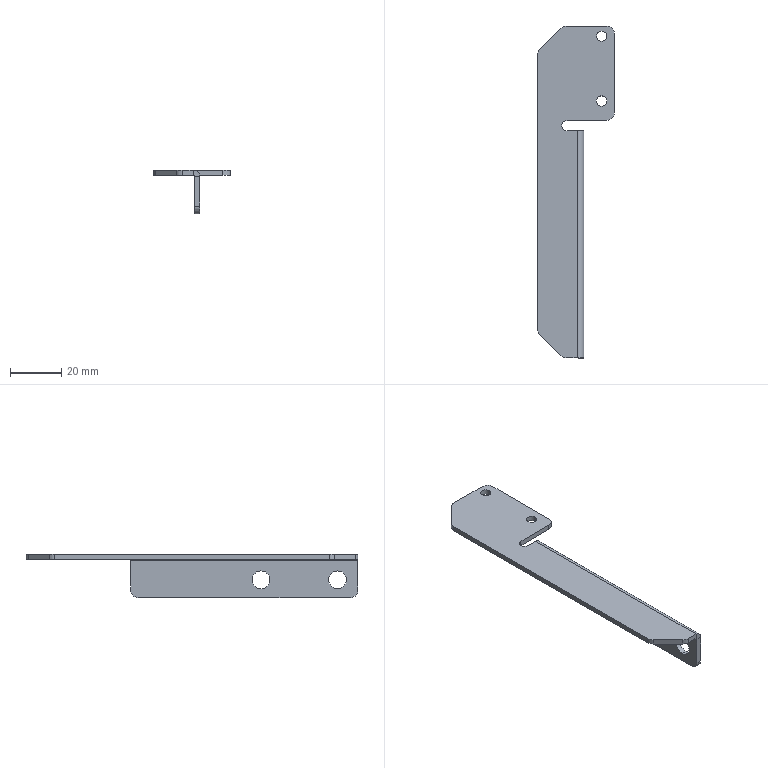Part | SolidWorks | features HoleWzd 2, EdgeFlange 1, Fillet 1, FlatPattern 1, SMBaseFlange 1, SheetMetal 1 | 1 solid | 36 faces | box 30 x 130 x 17 mm | volume 7638 mm3 | cylinder 19 | plane 17 | commonest cylinder face diameters 6 x8 4 x5 7 x4 1 x1 5 x1
STEP:
#1=CARTESIAN_POINT('',(23.,116.,-2.));
#2=VERTEX_POINT('',#1);
#3=CARTESIAN_POINT('',(27.,116.,-2.));
#4=VERTEX_POINT('',#3);
#5=CARTESIAN_POINT('',(25.,116.,-2.));
#6=DIRECTION('',(0.,0.,1.));
#7=DIRECTION('',(1.,0.,0.));
#8=AXIS2_PLACEMENT_3D('',#5,#6,#7);
#9=CIRCLE('',#8,2.);
#10=EDGE_CURVE('',#2,#4,#9,.T.);
#11=ORIENTED_EDGE('',*,*,#10,.F.);
#12=CARTESIAN_POINT('',(23.,116.,0.));
#13=VERTEX_POINT('',#12);
#14=CARTESIAN_POINT('',(23.,116.,0.));
#15=DIRECTION('',(0.,0.,1.));
#16=VECTOR('',#15,1000.);
#17=LINE('',#14,#16);
#18=EDGE_CURVE('',#2,#13,#17,.T.);
#19=ORIENTED_EDGE('',*,*,#18,.T.);
#20=CARTESIAN_POINT('',(27.,116.,0.));
#21=VERTEX_POINT('',#20);
#22=CARTESIAN_POINT('',(25.,116.,0.));
#23=DIRECTION('',(0.,0.,1.));
#24=DIRECTION('',(1.,0.,0.));
#25=AXIS2_PLACEMENT_3D('',#22,#23,#24);
#26=CIRCLE('',#25,2.);
#27=EDGE_CURVE('',#13,#21,#26,.T.);
#28=ORIENTED_EDGE('',*,*,#27,.T.);
#29=CARTESIAN_POINT('',(27.,116.,0.));
#30=DIRECTION('',(0.,0.,1.));
#31=VECTOR('',#30,1000.);
#32=LINE('',#29,#31);
#33=EDGE_CURVE('',#4,#21,#32,.T.);
#34=ORIENTED_EDGE('',*,*,#33,.F.);
#35=EDGE_LOOP('',(#11,#19,#28,#34));
#36=FACE_OUTER_BOUND('',#35,.T.);
#37=CARTESIAN_POINT('',(25.,116.,0.));
#38=DIRECTION('',(0.,0.,1.));
#39=DIRECTION('',(1.,0.,0.));
#40=AXIS2_PLACEMENT_3D('',#37,#38,#39);
#41=CYLINDRICAL_SURFACE('',#40,2.);
#42=ADVANCED_FACE('',(#36),#41,.F.);
#43=CARTESIAN_POINT('',(23.,90.6,-2.));
#44=VERTEX_POINT('',#43);
#45=CARTESIAN_POINT('',(27.,90.6,-2.));
#46=VERTEX_POINT('',#45);
#47=CARTESIAN_POINT('',(25.,90.6,-2.));
#48=DIRECTION('',(0.,0.,1.));
#49=DIRECTION('',(1.,0.,0.));
#50=AXIS2_PLACEMENT_3D('',#47,#48,#49);
#51=CIRCLE('',#50,2.);
#52=EDGE_CURVE('',#44,#46,#51,.T.);
#53=ORIENTED_EDGE('',*,*,#52,.F.);
#54=CARTESIAN_POINT('',(23.,90.6,0.));
#55=VERTEX_POINT('',#54);
#56=CARTESIAN_POINT('',(23.,90.6,0.));
#57=DIRECTION('',(0.,0.,1.));
#58=VECTOR('',#57,1000.);
#59=LINE('',#56,#58);
#60=EDGE_CURVE('',#44,#55,#59,.T.);
#61=ORIENTED_EDGE('',*,*,#60,.T.);
#62=CARTESIAN_POINT('',(27.,90.6,0.));
#63=VERTEX_POINT('',#62);
#64=CARTESIAN_POINT('',(25.,90.6,0.));
#65=DIRECTION('',(0.,0.,1.));
#66=DIRECTION('',(1.,0.,0.));
#67=AXIS2_PLACEMENT_3D('',#64,#65,#66);
#68=CIRCLE('',#67,2.);
#69=EDGE_CURVE('',#55,#63,#68,.T.);
#70=ORIENTED_EDGE('',*,*,#69,.T.);
#71=CARTESIAN_POINT('',(27.,90.6,0.));
#72=DIRECTION('',(0.,0.,1.));
#73=VECTOR('',#72,1000.);
#74=LINE('',#71,#73);
#75=EDGE_CURVE('',#46,#63,#74,.T.);
#76=ORIENTED_EDGE('',*,*,#75,.F.);
#77=EDGE_LOOP('',(#53,#61,#70,#76));
#78=FACE_OUTER_BOUND('',#77,.T.);
#79=CARTESIAN_POINT('',(25.,90.6,0.));
#80=DIRECTION('',(0.,0.,1.));
#81=DIRECTION('',(1.,0.,0.));
#82=AXIS2_PLACEMENT_3D('',#79,#80,#81);
#83=CYLINDRICAL_SURFACE('',#82,2.);
#84=ADVANCED_FACE('',(#78),#83,.F.);
#85=CARTESIAN_POINT('',(18.,28.,-6.5));
#86=VERTEX_POINT('',#85);
#87=CARTESIAN_POINT('',(18.,28.,-13.5));
#88=VERTEX_POINT('',#87);
#89=CARTESIAN_POINT('',(18.,28.,-10.));
#90=DIRECTION('',(1.,0.,0.));
#91=DIRECTION('',(0.,0.,-1.));
#92=AXIS2_PLACEMENT_3D('',#89,#90,#91);
#93=CIRCLE('',#92,3.5);
#94=EDGE_CURVE('',#86,#88,#93,.T.);
#95=ORIENTED_EDGE('',*,*,#94,.T.);
#96=CARTESIAN_POINT('',(16.,28.,-13.5));
#97=VERTEX_POINT('',#96);
#98=CARTESIAN_POINT('',(16.,28.,-13.5));
#99=DIRECTION('',(-1.,0.,0.));
#100=VECTOR('',#99,1000.);
#101=LINE('',#98,#100);
#102=EDGE_CURVE('',#88,#97,#101,.T.);
#103=ORIENTED_EDGE('',*,*,#102,.T.);
#104=CARTESIAN_POINT('',(16.,28.,-6.5));
#105=VERTEX_POINT('',#104);
#106=CARTESIAN_POINT('',(16.,28.,-10.));
#107=DIRECTION('',(-1.,0.,0.));
#108=DIRECTION('',(0.,0.,1.));
#109=AXIS2_PLACEMENT_3D('',#106,#107,#108);
#110=CIRCLE('',#109,3.5);
#111=EDGE_CURVE('',#97,#105,#110,.T.);
#112=ORIENTED_EDGE('',*,*,#111,.T.);
#113=CARTESIAN_POINT('',(16.,28.,-6.5));
#114=DIRECTION('',(-1.,0.,0.));
#115=VECTOR('',#114,1000.);
#116=LINE('',#113,#115);
#117=EDGE_CURVE('',#86,#105,#116,.T.);
#118=ORIENTED_EDGE('',*,*,#117,.F.);
#119=EDGE_LOOP('',(#95,#103,#112,#118));
#120=FACE_OUTER_BOUND('',#119,.T.);
#121=CARTESIAN_POINT('',(16.,28.,-10.));
#122=DIRECTION('',(-1.,0.,0.));
#123=DIRECTION('',(0.,0.,1.));
#124=AXIS2_PLACEMENT_3D('',#121,#122,#123);
#125=CYLINDRICAL_SURFACE('',#124,3.5);
#126=ADVANCED_FACE('',(#120),#125,.F.);
#127=CARTESIAN_POINT('',(18.,-2.,-6.5));
#128=VERTEX_POINT('',#127);
#129=CARTESIAN_POINT('',(18.,-2.,-13.5));
#130=VERTEX_POINT('',#129);
#131=CARTESIAN_POINT('',(18.,-2.,-10.));
#132=DIRECTION('',(1.,0.,0.));
#133=DIRECTION('',(0.,0.,-1.));
#134=AXIS2_PLACEMENT_3D('',#131,#132,#133);
#135=CIRCLE('',#134,3.5);
#136=EDGE_CURVE('',#128,#130,#135,.T.);
#137=ORIENTED_EDGE('',*,*,#136,.T.);
#138=CARTESIAN_POINT('',(16.,-2.,-13.5));
#139=VERTEX_POINT('',#138);
#140=CARTESIAN_POINT('',(16.,-2.,-13.5));
#141=DIRECTION('',(-1.,0.,0.));
#142=VECTOR('',#141,1000.);
#143=LINE('',#140,#142);
#144=EDGE_CURVE('',#130,#139,#143,.T.);
#145=ORIENTED_EDGE('',*,*,#144,.T.);
#146=CARTESIAN_POINT('',(16.,-2.,-6.5));
#147=VERTEX_POINT('',#146);
#148=CARTESIAN_POINT('',(16.,-2.,-10.));
#149=DIRECTION('',(-1.,0.,0.));
#150=DIRECTION('',(0.,0.,1.));
#151=AXIS2_PLACEMENT_3D('',#148,#149,#150);
#152=CIRCLE('',#151,3.5);
#153=EDGE_CURVE('',#139,#147,#152,.T.);
#154=ORIENTED_EDGE('',*,*,#153,.T.);
#155=CARTESIAN_POINT('',(16.,-2.,-6.5));
#156=DIRECTION('',(-1.,0.,0.));
#157=VECTOR('',#156,1000.);
#158=LINE('',#155,#157);
#159=EDGE_CURVE('',#128,#147,#158,.T.);
#160=ORIENTED_EDGE('',*,*,#159,.F.);
#161=EDGE_LOOP('',(#137,#145,#154,#160));
#162=FACE_OUTER_BOUND('',#161,.T.);
#163=CARTESIAN_POINT('',(16.,-2.,-10.));
#164=DIRECTION('',(-1.,0.,0.));
#165=DIRECTION('',(0.,0.,1.));
#166=AXIS2_PLACEMENT_3D('',#163,#164,#165);
#167=CYLINDRICAL_SURFACE('',#166,3.5);
#168=ADVANCED_FACE('',(#162),#167,.F.);
#169=CARTESIAN_POINT('',(30.,86.,0.));
#170=VERTEX_POINT('',#169);
#171=CARTESIAN_POINT('',(30.,117.,0.));
#172=VERTEX_POINT('',#171);
#173=CARTESIAN_POINT('',(30.,120.,0.));
#174=DIRECTION('',(0.,1.,0.));
#175=VECTOR('',#174,1000.);
#176=LINE('',#173,#175);
#177=EDGE_CURVE('',#170,#172,#176,.T.);
#178=ORIENTED_EDGE('',*,*,#177,.F.);
#179=CARTESIAN_POINT('',(30.,86.,-2.));
#180=VERTEX_POINT('',#179);
#181=CARTESIAN_POINT('',(30.,86.,-2.));
#182=DIRECTION('',(0.,0.,-1.));
#183=VECTOR('',#182,1000.);
#184=LINE('',#181,#183);
#185=EDGE_CURVE('',#170,#180,#184,.T.);
#186=ORIENTED_EDGE('',*,*,#185,.T.);
#187=CARTESIAN_POINT('',(30.,117.,-2.));
#188=VERTEX_POINT('',#187);
#189=CARTESIAN_POINT('',(30.,120.,-2.));
#190=DIRECTION('',(0.,1.,0.));
#191=VECTOR('',#190,1000.);
#192=LINE('',#189,#191);
#193=EDGE_CURVE('',#180,#188,#192,.T.);
#194=ORIENTED_EDGE('',*,*,#193,.T.);
#195=CARTESIAN_POINT('',(30.,117.,-2.));
#196=DIRECTION('',(0.,0.,1.));
#197=VECTOR('',#196,1000.);
#198=LINE('',#195,#197);
#199=EDGE_CURVE('',#188,#172,#198,.T.);
#200=ORIENTED_EDGE('',*,*,#199,.T.);
#201=EDGE_LOOP('',(#178,#186,#194,#200));
#202=FACE_OUTER_BOUND('',#201,.T.);
#203=CARTESIAN_POINT('',(30.,120.,-2.));
#204=DIRECTION('',(1.,0.,0.));
#205=DIRECTION('',(0.,1.,0.));
#206=AXIS2_PLACEMENT_3D('',#203,#204,#205);
#207=PLANE('',#206);
#208=ADVANCED_FACE('',(#202),#207,.T.);
#209=CARTESIAN_POINT('',(11.243,-10.,0.));
#210=VERTEX_POINT('',#209);
#211=CARTESIAN_POINT('',(15.5,-10.,0.));
#212=VERTEX_POINT('',#211);
#213=CARTESIAN_POINT('',(10.,-10.,0.));
#214=DIRECTION('',(1.,0.,0.));
#215=VECTOR('',#214,1000.);
#216=LINE('',#213,#215);
#217=EDGE_CURVE('',#210,#212,#216,.T.);
#218=ORIENTED_EDGE('',*,*,#217,.F.);
#219=CARTESIAN_POINT('',(11.243,-10.,-2.));
#220=VERTEX_POINT('',#219);
#221=CARTESIAN_POINT('',(11.243,-10.,-2.));
#222=DIRECTION('',(0.,0.,-1.));
#223=VECTOR('',#222,1000.);
#224=LINE('',#221,#223);
#225=EDGE_CURVE('',#210,#220,#224,.T.);
#226=ORIENTED_EDGE('',*,*,#225,.T.);
#227=CARTESIAN_POINT('',(15.5,-10.,-2.));
#228=VERTEX_POINT('',#227);
#229=CARTESIAN_POINT('',(10.,-10.,-2.));
#230=DIRECTION('',(1.,0.,0.));
#231=VECTOR('',#230,1000.);
#232=LINE('',#229,#231);
#233=EDGE_CURVE('',#220,#228,#232,.T.);
#234=ORIENTED_EDGE('',*,*,#233,.T.);
#235=CARTESIAN_POINT('',(15.5,-10.,-2.));
#236=DIRECTION('',(0.,0.,1.));
#237=VECTOR('',#236,1000.);
#238=LINE('',#235,#237);
#239=EDGE_CURVE('',#228,#212,#238,.T.);
#240=ORIENTED_EDGE('',*,*,#239,.T.);
#241=EDGE_LOOP('',(#218,#226,#234,#240));
#242=FACE_OUTER_BOUND('',#241,.T.);
#243=CARTESIAN_POINT('',(10.,-10.,-2.));
#244=DIRECTION('',(0.,-1.,0.));
#245=DIRECTION('',(1.,0.,0.));
#246=AXIS2_PLACEMENT_3D('',#243,#244,#245);
#247=PLANE('',#246);
#248=ADVANCED_FACE('',(#242),#247,.T.);
#249=CARTESIAN_POINT('',(25.,116.,-2.));
#250=DIRECTION('',(0.,0.,1.));
#251=DIRECTION('',(1.,0.,0.));
#252=AXIS2_PLACEMENT_3D('',#249,#250,#251);
#253=CIRCLE('',#252,2.);
#254=EDGE_CURVE('',#4,#2,#253,.T.);
#255=ORIENTED_EDGE('',*,*,#254,.T.);
#256=ORIENTED_EDGE('',*,*,#10,.T.);
#257=EDGE_LOOP('',(#255,#256));
#258=FACE_BOUND('',#257,.T.);
#259=CARTESIAN_POINT('',(25.,90.6,-2.));
#260=DIRECTION('',(0.,0.,1.));
#261=DIRECTION('',(1.,0.,0.));
#262=AXIS2_PLACEMENT_3D('',#259,#260,#261);
#263=CIRCLE('',#262,2.);
#264=EDGE_CURVE('',#46,#44,#263,.T.);
#265=ORIENTED_EDGE('',*,*,#264,.T.);
#266=ORIENTED_EDGE('',*,*,#52,.T.);
#267=EDGE_LOOP('',(#265,#266));
#268=FACE_BOUND('',#267,.T.);
#269=ORIENTED_EDGE('',*,*,#193,.F.);
#270=CARTESIAN_POINT('',(27.,83.,-2.));
#271=VERTEX_POINT('',#270);
#272=CARTESIAN_POINT('',(27.,86.,-2.));
#273=DIRECTION('',(0.,0.,-1.));
#274=DIRECTION('',(1.,0.,0.));
#275=AXIS2_PLACEMENT_3D('',#272,#273,#274);
#276=CIRCLE('',#275,3.);
#277=EDGE_CURVE('',#180,#271,#276,.T.);
#278=ORIENTED_EDGE('',*,*,#277,.T.);
#279=CARTESIAN_POINT('',(11.5,83.,-2.));
#280=VERTEX_POINT('',#279);
#281=CARTESIAN_POINT('',(11.5,83.,-2.));
#282=DIRECTION('',(1.,0.,0.));
#283=VECTOR('',#282,1000.);
#284=LINE('',#281,#283);
#285=EDGE_CURVE('',#280,#271,#284,.T.);
#286=ORIENTED_EDGE('',*,*,#285,.F.);
#287=CARTESIAN_POINT('',(11.5,79.,-2.));
#288=VERTEX_POINT('',#287);
#289=CARTESIAN_POINT('',(11.5,81.,-2.));
#290=DIRECTION('',(0.,0.,-1.));
#291=DIRECTION('',(-1.,0.,0.));
#292=AXIS2_PLACEMENT_3D('',#289,#290,#291);
#293=CIRCLE('',#292,2.);
#294=EDGE_CURVE('',#288,#280,#293,.T.);
#295=ORIENTED_EDGE('',*,*,#294,.F.);
#296=CARTESIAN_POINT('',(15.5,79.,-2.));
#297=VERTEX_POINT('',#296);
#298=CARTESIAN_POINT('',(15.5,79.,-2.));
#299=DIRECTION('',(-1.,0.,0.));
#300=VECTOR('',#299,1000.);
#301=LINE('',#298,#300);
#302=EDGE_CURVE('',#297,#288,#301,.T.);
#303=ORIENTED_EDGE('',*,*,#302,.F.);
#304=CARTESIAN_POINT('',(15.5,-10.,-2.));
#305=DIRECTION('',(0.,1.,0.));
#306=VECTOR('',#305,1000.);
#307=LINE('',#304,#306);
#308=EDGE_CURVE('',#228,#297,#307,.T.);
#309=ORIENTED_EDGE('',*,*,#308,.F.);
#310=ORIENTED_EDGE('',*,*,#233,.F.);
#311=CARTESIAN_POINT('',(9.121,-9.121,-2.));
#312=VERTEX_POINT('',#311);
#313=CARTESIAN_POINT('',(11.243,-7.,-2.));
#314=DIRECTION('',(0.,0.,-1.));
#315=DIRECTION('',(1.,0.,0.));
#316=AXIS2_PLACEMENT_3D('',#313,#314,#315);
#317=CIRCLE('',#316,3.);
#318=EDGE_CURVE('',#220,#312,#317,.T.);
#319=ORIENTED_EDGE('',*,*,#318,.T.);
#320=CARTESIAN_POINT('',(0.8787,-0.8787,-2.));
#321=VERTEX_POINT('',#320);
#322=CARTESIAN_POINT('',(0.,0.,-2.));
#323=DIRECTION('',(0.7071,-0.7071,0.));
#324=VECTOR('',#323,1000.);
#325=LINE('',#322,#324);
#326=EDGE_CURVE('',#321,#312,#325,.T.);
#327=ORIENTED_EDGE('',*,*,#326,.F.);
#328=CARTESIAN_POINT('',(0.,1.243,-2.));
#329=VERTEX_POINT('',#328);
#330=CARTESIAN_POINT('',(3.,1.243,-2.));
#331=DIRECTION('',(0.,0.,-1.));
#332=DIRECTION('',(1.,0.,0.));
#333=AXIS2_PLACEMENT_3D('',#330,#331,#332);
#334=CIRCLE('',#333,3.);
#335=EDGE_CURVE('',#321,#329,#334,.T.);
#336=ORIENTED_EDGE('',*,*,#335,.T.);
#337=CARTESIAN_POINT('',(0.,108.757,-2.));
#338=VERTEX_POINT('',#337);
#339=CARTESIAN_POINT('',(0.,0.,-2.));
#340=DIRECTION('',(0.,-1.,0.));
#341=VECTOR('',#340,1000.);
#342=LINE('',#339,#341);
#343=EDGE_CURVE('',#338,#329,#342,.T.);
#344=ORIENTED_EDGE('',*,*,#343,.F.);
#345=CARTESIAN_POINT('',(0.8787,110.879,-2.));
#346=VERTEX_POINT('',#345);
#347=CARTESIAN_POINT('',(3.,108.757,-2.));
#348=DIRECTION('',(0.,0.,-1.));
#349=DIRECTION('',(1.,0.,0.));
#350=AXIS2_PLACEMENT_3D('',#347,#348,#349);
#351=CIRCLE('',#350,3.);
#352=EDGE_CURVE('',#338,#346,#351,.T.);
#353=ORIENTED_EDGE('',*,*,#352,.T.);
#354=CARTESIAN_POINT('',(9.121,119.121,-2.));
#355=VERTEX_POINT('',#354);
#356=CARTESIAN_POINT('',(0.,110.,-2.));
#357=DIRECTION('',(-0.7071,-0.7071,0.));
#358=VECTOR('',#357,1000.);
#359=LINE('',#356,#358);
#360=EDGE_CURVE('',#355,#346,#359,.T.);
#361=ORIENTED_EDGE('',*,*,#360,.F.);
#362=CARTESIAN_POINT('',(11.243,120.,-2.));
#363=VERTEX_POINT('',#362);
#364=CARTESIAN_POINT('',(11.243,117.,-2.));
#365=DIRECTION('',(0.,0.,-1.));
#366=DIRECTION('',(1.,0.,0.));
#367=AXIS2_PLACEMENT_3D('',#364,#365,#366);
#368=CIRCLE('',#367,3.);
#369=EDGE_CURVE('',#355,#363,#368,.T.);
#370=ORIENTED_EDGE('',*,*,#369,.T.);
#371=CARTESIAN_POINT('',(27.,120.,-2.));
#372=VERTEX_POINT('',#371);
#373=CARTESIAN_POINT('',(10.,120.,-2.));
#374=DIRECTION('',(-1.,0.,0.));
#375=VECTOR('',#374,1000.);
#376=LINE('',#373,#375);
#377=EDGE_CURVE('',#372,#363,#376,.T.);
#378=ORIENTED_EDGE('',*,*,#377,.F.);
#379=CARTESIAN_POINT('',(27.,117.,-2.));
#380=DIRECTION('',(0.,0.,-1.));
#381=DIRECTION('',(1.,0.,0.));
#382=AXIS2_PLACEMENT_3D('',#379,#380,#381);
#383=CIRCLE('',#382,3.);
#384=EDGE_CURVE('',#372,#188,#383,.T.);
#385=ORIENTED_EDGE('',*,*,#384,.T.);
#386=EDGE_LOOP('',(#269,#278,#286,#295,#303,#309,#310,#319,#327,#336,#344,#353,#361,#370,#378,#385));
#387=FACE_OUTER_BOUND('',#386,.T.);
#388=CARTESIAN_POINT('',(0.,0.,-2.));
#389=DIRECTION('',(0.,0.,1.));
#390=DIRECTION('',(1.,0.,0.));
#391=AXIS2_PLACEMENT_3D('',#388,#389,#390);
#392=PLANE('',#391);
#393=ADVANCED_FACE('',(#258,#268,#387),#392,.F.);
#394=CARTESIAN_POINT('',(25.,116.,0.));
#395=DIRECTION('',(0.,0.,1.));
#396=DIRECTION('',(1.,0.,0.));
#397=AXIS2_PLACEMENT_3D('',#394,#395,#396);
#398=CIRCLE('',#397,2.);
#399=EDGE_CURVE('',#21,#13,#398,.T.);
#400=ORIENTED_EDGE('',*,*,#399,.F.);
#401=ORIENTED_EDGE('',*,*,#27,.F.);
#402=EDGE_LOOP('',(#400,#401));
#403=FACE_BOUND('',#402,.T.);
#404=CARTESIAN_POINT('',(25.,90.6,0.));
#405=DIRECTION('',(0.,0.,1.));
#406=DIRECTION('',(1.,0.,0.));
#407=AXIS2_PLACEMENT_3D('',#404,#405,#406);
#408=CIRCLE('',#407,2.);
#409=EDGE_CURVE('',#63,#55,#408,.T.);
#410=ORIENTED_EDGE('',*,*,#409,.F.);
#411=ORIENTED_EDGE('',*,*,#69,.F.);
#412=EDGE_LOOP('',(#410,#411));
#413=FACE_BOUND('',#412,.T.);
#414=CARTESIAN_POINT('',(11.5,83.,0.));
#415=VERTEX_POINT('',#414);
#416=CARTESIAN_POINT('',(27.,83.,0.));
#417=VERTEX_POINT('',#416);
#418=CARTESIAN_POINT('',(0.,83.,0.));
#419=DIRECTION('',(1.,0.,0.));
#420=VECTOR('',#419,1000.);
#421=LINE('',#418,#420);
#422=EDGE_CURVE('',#415,#417,#421,.T.);
#423=ORIENTED_EDGE('',*,*,#422,.T.);
#424=CARTESIAN_POINT('',(27.,86.,0.));
#425=DIRECTION('',(0.,0.,1.));
#426=DIRECTION('',(1.,0.,0.));
#427=AXIS2_PLACEMENT_3D('',#424,#425,#426);
#428=CIRCLE('',#427,3.);
#429=EDGE_CURVE('',#417,#170,#428,.T.);
#430=ORIENTED_EDGE('',*,*,#429,.T.);
#431=ORIENTED_EDGE('',*,*,#177,.T.);
#432=CARTESIAN_POINT('',(27.,120.,0.));
#433=VERTEX_POINT('',#432);
#434=CARTESIAN_POINT('',(27.,117.,0.));
#435=DIRECTION('',(0.,0.,1.));
#436=DIRECTION('',(1.,0.,0.));
#437=AXIS2_PLACEMENT_3D('',#434,#435,#436);
#438=CIRCLE('',#437,3.);
#439=EDGE_CURVE('',#172,#433,#438,.T.);
#440=ORIENTED_EDGE('',*,*,#439,.T.);
#441=CARTESIAN_POINT('',(11.243,120.,0.));
#442=VERTEX_POINT('',#441);
#443=CARTESIAN_POINT('',(10.,120.,0.));
#444=DIRECTION('',(-1.,0.,0.));
#445=VECTOR('',#444,1000.);
#446=LINE('',#443,#445);
#447=EDGE_CURVE('',#433,#442,#446,.T.);
#448=ORIENTED_EDGE('',*,*,#447,.T.);
#449=CARTESIAN_POINT('',(9.121,119.121,0.));
#450=VERTEX_POINT('',#449);
#451=CARTESIAN_POINT('',(11.243,117.,0.));
#452=DIRECTION('',(0.,0.,1.));
#453=DIRECTION('',(1.,0.,0.));
#454=AXIS2_PLACEMENT_3D('',#451,#452,#453);
#455=CIRCLE('',#454,3.);
#456=EDGE_CURVE('',#442,#450,#455,.T.);
#457=ORIENTED_EDGE('',*,*,#456,.T.);
#458=CARTESIAN_POINT('',(0.8787,110.879,0.));
#459=VERTEX_POINT('',#458);
#460=CARTESIAN_POINT('',(0.,110.,0.));
#461=DIRECTION('',(-0.7071,-0.7071,0.));
#462=VECTOR('',#461,1000.);
#463=LINE('',#460,#462);
#464=EDGE_CURVE('',#450,#459,#463,.T.);
#465=ORIENTED_EDGE('',*,*,#464,.T.);
#466=CARTESIAN_POINT('',(0.,108.757,0.));
#467=VERTEX_POINT('',#466);
#468=CARTESIAN_POINT('',(3.,108.757,0.));
#469=DIRECTION('',(0.,0.,1.));
#470=DIRECTION('',(1.,0.,0.));
#471=AXIS2_PLACEMENT_3D('',#468,#469,#470);
#472=CIRCLE('',#471,3.);
#473=EDGE_CURVE('',#459,#467,#472,.T.);
#474=ORIENTED_EDGE('',*,*,#473,.T.);
#475=CARTESIAN_POINT('',(0.,1.243,0.));
#476=VERTEX_POINT('',#475);
#477=CARTESIAN_POINT('',(0.,0.,0.));
#478=DIRECTION('',(0.,-1.,0.));
#479=VECTOR('',#478,1000.);
#480=LINE('',#477,#479);
#481=EDGE_CURVE('',#467,#476,#480,.T.);
#482=ORIENTED_EDGE('',*,*,#481,.T.);
#483=CARTESIAN_POINT('',(0.8787,-0.8787,0.));
#484=VERTEX_POINT('',#483);
#485=CARTESIAN_POINT('',(3.,1.243,0.));
#486=DIRECTION('',(0.,0.,1.));
#487=DIRECTION('',(1.,0.,0.));
#488=AXIS2_PLACEMENT_3D('',#485,#486,#487);
#489=CIRCLE('',#488,3.);
#490=EDGE_CURVE('',#476,#484,#489,.T.);
#491=ORIENTED_EDGE('',*,*,#490,.T.);
#492=CARTESIAN_POINT('',(9.121,-9.121,0.));
#493=VERTEX_POINT('',#492);
#494=CARTESIAN_POINT('',(0.,0.,0.));
#495=DIRECTION('',(0.7071,-0.7071,0.));
#496=VECTOR('',#495,1000.);
#497=LINE('',#494,#496);
#498=EDGE_CURVE('',#484,#493,#497,.T.);
#499=ORIENTED_EDGE('',*,*,#498,.T.);
#500=CARTESIAN_POINT('',(11.243,-7.,0.));
#501=DIRECTION('',(0.,0.,1.));
#502=DIRECTION('',(1.,0.,0.));
#503=AXIS2_PLACEMENT_3D('',#500,#501,#502);
#504=CIRCLE('',#503,3.);
#505=EDGE_CURVE('',#493,#210,#504,.T.);
#506=ORIENTED_EDGE('',*,*,#505,.T.);
#507=ORIENTED_EDGE('',*,*,#217,.T.);
#508=CARTESIAN_POINT('',(15.5,79.,0.));
#509=VERTEX_POINT('',#508);
#510=CARTESIAN_POINT('',(15.5,-10.,0.));
#511=DIRECTION('',(0.,1.,0.));
#512=VECTOR('',#511,1000.);
#513=LINE('',#510,#512);
#514=EDGE_CURVE('',#212,#509,#513,.T.);
#515=ORIENTED_EDGE('',*,*,#514,.T.);
#516=CARTESIAN_POINT('',(11.5,79.,0.));
#517=VERTEX_POINT('',#516);
#518=CARTESIAN_POINT('',(0.,79.,0.));
#519=DIRECTION('',(-1.,0.,0.));
#520=VECTOR('',#519,1000.);
#521=LINE('',#518,#520);
#522=EDGE_CURVE('',#509,#517,#521,.T.);
#523=ORIENTED_EDGE('',*,*,#522,.T.);
#524=CARTESIAN_POINT('',(11.5,81.,0.));
#525=DIRECTION('',(0.,0.,-1.));
#526=DIRECTION('',(1.,0.,0.));
#527=AXIS2_PLACEMENT_3D('',#524,#525,#526);
#528=CIRCLE('',#527,2.);
#529=EDGE_CURVE('',#517,#415,#528,.T.);
#530=ORIENTED_EDGE('',*,*,#529,.T.);
#531=EDGE_LOOP('',(#423,#430,#431,#440,#448,#457,#465,#474,#482,#491,#499,#506,#507,#515,#523,#530));
#532=FACE_OUTER_BOUND('',#531,.T.);
#533=CARTESIAN_POINT('',(0.,0.,0.));
#534=DIRECTION('',(0.,0.,1.));
#535=DIRECTION('',(1.,0.,0.));
#536=AXIS2_PLACEMENT_3D('',#533,#534,#535);
#537=PLANE('',#536);
#538=ADVANCED_FACE('',(#403,#413,#532),#537,.T.);
#539=ORIENTED_EDGE('',*,*,#498,.F.);
#540=CARTESIAN_POINT('',(0.8787,-0.8787,-2.));
#541=DIRECTION('',(0.,0.,-1.));
#542=VECTOR('',#541,1000.);
#543=LINE('',#540,#542);
#544=EDGE_CURVE('',#484,#321,#543,.T.);
#545=ORIENTED_EDGE('',*,*,#544,.T.);
#546=ORIENTED_EDGE('',*,*,#326,.T.);
#547=CARTESIAN_POINT('',(9.121,-9.121,-2.));
#548=DIRECTION('',(0.,0.,1.));
#549=VECTOR('',#548,1000.);
#550=LINE('',#547,#549);
#551=EDGE_CURVE('',#312,#493,#550,.T.);
#552=ORIENTED_EDGE('',*,*,#551,.T.);
#553=EDGE_LOOP('',(#539,#545,#546,#552));
#554=FACE_OUTER_BOUND('',#553,.T.);
#555=CARTESIAN_POINT('',(0.,0.,-2.));
#556=DIRECTION('',(-0.7071,-0.7071,0.));
#557=DIRECTION('',(0.7071,-0.7071,0.));
#558=AXIS2_PLACEMENT_3D('',#555,#556,#557);
#559=PLANE('',#558);
#560=ADVANCED_FACE('',(#554),#559,.T.);
#561=ORIENTED_EDGE('',*,*,#343,.T.);
#562=CARTESIAN_POINT('',(0.,1.243,-2.));
#563=DIRECTION('',(0.,0.,1.));
#564=VECTOR('',#563,1000.);
#565=LINE('',#562,#564);
#566=EDGE_CURVE('',#329,#476,#565,.T.);
#567=ORIENTED_EDGE('',*,*,#566,.T.);
#568=ORIENTED_EDGE('',*,*,#481,.F.);
#569=CARTESIAN_POINT('',(0.,108.757,-2.));
#570=DIRECTION('',(0.,0.,-1.));
#571=VECTOR('',#570,1000.);
#572=LINE('',#569,#571);
#573=EDGE_CURVE('',#467,#338,#572,.T.);
#574=ORIENTED_EDGE('',*,*,#573,.T.);
#575=EDGE_LOOP('',(#561,#567,#568,#574));
#576=FACE_OUTER_BOUND('',#575,.T.);
#577=CARTESIAN_POINT('',(0.,0.,-2.));
#578=DIRECTION('',(-1.,0.,0.));
#579=DIRECTION('',(0.,0.,1.));
#580=AXIS2_PLACEMENT_3D('',#577,#578,#579);
#581=PLANE('',#580);
#582=ADVANCED_FACE('',(#576),#581,.T.);
#583=ORIENTED_EDGE('',*,*,#360,.T.);
#584=CARTESIAN_POINT('',(0.8787,110.879,-2.));
#585=DIRECTION('',(0.,0.,1.));
#586=VECTOR('',#585,1000.);
#587=LINE('',#584,#586);
#588=EDGE_CURVE('',#346,#459,#587,.T.);
#589=ORIENTED_EDGE('',*,*,#588,.T.);
#590=ORIENTED_EDGE('',*,*,#464,.F.);
#591=CARTESIAN_POINT('',(9.121,119.121,-2.));
#592=DIRECTION('',(0.,0.,-1.));
#593=VECTOR('',#592,1000.);
#594=LINE('',#591,#593);
#595=EDGE_CURVE('',#450,#355,#594,.T.);
#596=ORIENTED_EDGE('',*,*,#595,.T.);
#597=EDGE_LOOP('',(#583,#589,#590,#596));
#598=FACE_OUTER_BOUND('',#597,.T.);
#599=CARTESIAN_POINT('',(0.,110.,-2.));
#600=DIRECTION('',(-0.7071,0.7071,0.));
#601=DIRECTION('',(-0.7071,-0.7071,0.));
#602=AXIS2_PLACEMENT_3D('',#599,#600,#601);
#603=PLANE('',#602);
#604=ADVANCED_FACE('',(#598),#603,.T.);
#605=ORIENTED_EDGE('',*,*,#377,.T.);
#606=CARTESIAN_POINT('',(11.243,120.,-2.));
#607=DIRECTION('',(0.,0.,1.));
#608=VECTOR('',#607,1000.);
#609=LINE('',#606,#608);
#610=EDGE_CURVE('',#363,#442,#609,.T.);
#611=ORIENTED_EDGE('',*,*,#610,.T.);
#612=ORIENTED_EDGE('',*,*,#447,.F.);
#613=CARTESIAN_POINT('',(27.,120.,-2.));
#614=DIRECTION('',(0.,0.,-1.));
#615=VECTOR('',#614,1000.);
#616=LINE('',#613,#615);
#617=EDGE_CURVE('',#433,#372,#616,.T.);
#618=ORIENTED_EDGE('',*,*,#617,.T.);
#619=EDGE_LOOP('',(#605,#611,#612,#618));
#620=FACE_OUTER_BOUND('',#619,.T.);
#621=CARTESIAN_POINT('',(10.,120.,-2.));
#622=DIRECTION('',(0.,1.,0.));
#623=DIRECTION('',(0.,0.,1.));
#624=AXIS2_PLACEMENT_3D('',#621,#622,#623);
#625=PLANE('',#624);
#626=ADVANCED_FACE('',(#620),#625,.T.);
#627=ORIENTED_EDGE('',*,*,#522,.F.);
#628=CARTESIAN_POINT('',(15.5,79.,-2.));
#629=DIRECTION('',(0.,0.,1.));
#630=VECTOR('',#629,1000.);
#631=LINE('',#628,#630);
#632=EDGE_CURVE('',#297,#509,#631,.T.);
#633=ORIENTED_EDGE('',*,*,#632,.F.);
#634=ORIENTED_EDGE('',*,*,#302,.T.);
#635=CARTESIAN_POINT('',(11.5,79.,-2.));
#636=DIRECTION('',(0.,0.,1.));
#637=VECTOR('',#636,1000.);
#638=LINE('',#635,#637);
#639=EDGE_CURVE('',#288,#517,#638,.T.);
#640=ORIENTED_EDGE('',*,*,#639,.T.);
#641=EDGE_LOOP('',(#627,#633,#634,#640));
#642=FACE_OUTER_BOUND('',#641,.T.);
#643=CARTESIAN_POINT('',(15.5,79.,-2.));
#644=DIRECTION('',(0.,1.,0.));
#645=DIRECTION('',(0.,0.,1.));
#646=AXIS2_PLACEMENT_3D('',#643,#644,#645);
#647=PLANE('',#646);
#648=ADVANCED_FACE('',(#642),#647,.T.);
#649=ORIENTED_EDGE('',*,*,#529,.F.);
#650=ORIENTED_EDGE('',*,*,#639,.F.);
#651=ORIENTED_EDGE('',*,*,#294,.T.);
#652=CARTESIAN_POINT('',(11.5,83.,-2.));
#653=DIRECTION('',(0.,0.,1.));
#654=VECTOR('',#653,1000.);
#655=LINE('',#652,#654);
#656=EDGE_CURVE('',#280,#415,#655,.T.);
#657=ORIENTED_EDGE('',*,*,#656,.T.);
#658=EDGE_LOOP('',(#649,#650,#651,#657));
#659=FACE_OUTER_BOUND('',#658,.T.);
#660=CARTESIAN_POINT('',(11.5,81.,-2.));
#661=DIRECTION('',(0.,0.,1.));
#662=DIRECTION('',(1.,0.,0.));
#663=AXIS2_PLACEMENT_3D('',#660,#661,#662);
#664=CYLINDRICAL_SURFACE('',#663,2.);
#665=ADVANCED_FACE('',(#659),#664,.F.);
#666=ORIENTED_EDGE('',*,*,#285,.T.);
#667=CARTESIAN_POINT('',(27.,83.,-2.));
#668=DIRECTION('',(0.,0.,1.));
#669=VECTOR('',#668,1000.);
#670=LINE('',#667,#669);
#671=EDGE_CURVE('',#271,#417,#670,.T.);
#672=ORIENTED_EDGE('',*,*,#671,.T.);
#673=ORIENTED_EDGE('',*,*,#422,.F.);
#674=ORIENTED_EDGE('',*,*,#656,.F.);
#675=EDGE_LOOP('',(#666,#672,#673,#674));
#676=FACE_OUTER_BOUND('',#675,.T.);
#677=CARTESIAN_POINT('',(11.5,83.,-2.));
#678=DIRECTION('',(0.,-1.,0.));
#679=DIRECTION('',(0.,0.,-1.));
#680=AXIS2_PLACEMENT_3D('',#677,#678,#679);
#681=PLANE('',#680);
#682=ADVANCED_FACE('',(#676),#681,.T.);
#683=CARTESIAN_POINT('',(16.,79.,-2.5));
#684=VERTEX_POINT('',#683);
#685=CARTESIAN_POINT('',(18.,79.,-2.5));
#686=VERTEX_POINT('',#685);
#687=CARTESIAN_POINT('',(18.,79.,-2.5));
#688=DIRECTION('',(1.,0.,0.));
#689=VECTOR('',#688,1000.);
#690=LINE('',#687,#689);
#691=EDGE_CURVE('',#684,#686,#690,.T.);
#692=ORIENTED_EDGE('',*,*,#691,.F.);
#693=CARTESIAN_POINT('',(15.5,79.,-2.5));
#694=DIRECTION('',(0.,1.,0.));
#695=DIRECTION('',(0.,0.,-1.));
#696=AXIS2_PLACEMENT_3D('',#693,#694,#695);
#697=CIRCLE('',#696,0.5);
#698=EDGE_CURVE('',#297,#684,#697,.T.);
#699=ORIENTED_EDGE('',*,*,#698,.F.);
#700=ORIENTED_EDGE('',*,*,#632,.T.);
#701=CARTESIAN_POINT('',(15.5,79.,-2.5));
#702=DIRECTION('',(0.,1.,0.));
#703=DIRECTION('',(0.,0.,-1.));
#704=AXIS2_PLACEMENT_3D('',#701,#702,#703);
#705=CIRCLE('',#704,2.5);
#706=EDGE_CURVE('',#509,#686,#705,.T.);
#707=ORIENTED_EDGE('',*,*,#706,.T.);
#708=EDGE_LOOP('',(#692,#699,#700,#707));
#709=FACE_OUTER_BOUND('',#708,.T.);
#710=CARTESIAN_POINT('',(15.5,79.,-2.5));
#711=DIRECTION('',(0.,1.,0.));
#712=DIRECTION('',(0.,0.,1.));
#713=AXIS2_PLACEMENT_3D('',#710,#711,#712);
#714=PLANE('',#713);
#715=ADVANCED_FACE('',(#709),#714,.T.);
#716=CARTESIAN_POINT('',(16.,-10.,-2.5));
#717=VERTEX_POINT('',#716);
#718=CARTESIAN_POINT('',(15.5,-10.,-2.5));
#719=DIRECTION('',(0.,-1.,0.));
#720=DIRECTION('',(0.,0.,-1.));
#721=AXIS2_PLACEMENT_3D('',#718,#719,#720);
#722=CIRCLE('',#721,0.5);
#723=EDGE_CURVE('',#717,#228,#722,.T.);
#724=ORIENTED_EDGE('',*,*,#723,.F.);
#725=CARTESIAN_POINT('',(18.,-10.,-2.5));
#726=VERTEX_POINT('',#725);
#727=CARTESIAN_POINT('',(16.,-10.,-2.5));
#728=DIRECTION('',(1.,0.,0.));
#729=VECTOR('',#728,1000.);
#730=LINE('',#727,#729);
#731=EDGE_CURVE('',#717,#726,#730,.T.);
#732=ORIENTED_EDGE('',*,*,#731,.T.);
#733=CARTESIAN_POINT('',(15.5,-10.,-2.5));
#734=DIRECTION('',(0.,-1.,0.));
#735=DIRECTION('',(0.,0.,-1.));
#736=AXIS2_PLACEMENT_3D('',#733,#734,#735);
#737=CIRCLE('',#736,2.5);
#738=EDGE_CURVE('',#726,#212,#737,.T.);
#739=ORIENTED_EDGE('',*,*,#738,.T.);
#740=ORIENTED_EDGE('',*,*,#239,.F.);
#741=EDGE_LOOP('',(#724,#732,#739,#740));
#742=FACE_OUTER_BOUND('',#741,.T.);
#743=CARTESIAN_POINT('',(15.5,-10.,-2.5));
#744=DIRECTION('',(0.,1.,0.));
#745=DIRECTION('',(0.,0.,1.));
#746=AXIS2_PLACEMENT_3D('',#743,#744,#745);
#747=PLANE('',#746);
#748=ADVANCED_FACE('',(#742),#747,.F.);
#749=ORIENTED_EDGE('',*,*,#514,.F.);
#750=ORIENTED_EDGE('',*,*,#738,.F.);
#751=CARTESIAN_POINT('',(18.,0.,-2.5));
#752=DIRECTION('',(0.,-1.,0.));
#753=VECTOR('',#752,1000.);
#754=LINE('',#751,#753);
#755=EDGE_CURVE('',#686,#726,#754,.T.);
#756=ORIENTED_EDGE('',*,*,#755,.F.);
#757=ORIENTED_EDGE('',*,*,#706,.F.);
#758=EDGE_LOOP('',(#749,#750,#756,#757));
#759=FACE_OUTER_BOUND('',#758,.T.);
#760=CARTESIAN_POINT('',(15.5,-10.,-2.5));
#761=DIRECTION('',(0.,-1.,0.));
#762=DIRECTION('',(1.,0.,0.));
#763=AXIS2_PLACEMENT_3D('',#760,#761,#762);
#764=CYLINDRICAL_SURFACE('',#763,2.5);
#765=ADVANCED_FACE('',(#759),#764,.T.);
#766=ORIENTED_EDGE('',*,*,#308,.T.);
#767=ORIENTED_EDGE('',*,*,#698,.T.);
#768=CARTESIAN_POINT('',(16.,79.,-2.5));
#769=DIRECTION('',(0.,-1.,0.));
#770=VECTOR('',#769,1000.);
#771=LINE('',#768,#770);
#772=EDGE_CURVE('',#684,#717,#771,.T.);
#773=ORIENTED_EDGE('',*,*,#772,.T.);
#774=ORIENTED_EDGE('',*,*,#723,.T.);
#775=EDGE_LOOP('',(#766,#767,#773,#774));
#776=FACE_OUTER_BOUND('',#775,.T.);
#777=CARTESIAN_POINT('',(15.5,-10.,-2.5));
#778=DIRECTION('',(0.,-1.,0.));
#779=DIRECTION('',(1.,0.,0.));
#780=AXIS2_PLACEMENT_3D('',#777,#778,#779);
#781=CYLINDRICAL_SURFACE('',#780,0.5);
#782=ADVANCED_FACE('',(#776),#781,.F.);
#783=CARTESIAN_POINT('',(16.,-10.,-14.));
#784=VERTEX_POINT('',#783);
#785=CARTESIAN_POINT('',(16.,-10.,0.));
#786=DIRECTION('',(0.,0.,1.));
#787=VECTOR('',#786,1000.);
#788=LINE('',#785,#787);
#789=EDGE_CURVE('',#784,#717,#788,.T.);
#790=ORIENTED_EDGE('',*,*,#789,.F.);
#791=CARTESIAN_POINT('',(18.,-10.,-14.));
#792=VERTEX_POINT('',#791);
#793=CARTESIAN_POINT('',(18.,-10.,-14.));
#794=DIRECTION('',(1.,0.,0.));
#795=VECTOR('',#794,1000.);
#796=LINE('',#793,#795);
#797=EDGE_CURVE('',#784,#792,#796,.T.);
#798=ORIENTED_EDGE('',*,*,#797,.T.);
#799=CARTESIAN_POINT('',(18.,-10.,-2.));
#800=DIRECTION('',(0.,0.,1.));
#801=VECTOR('',#800,1000.);
#802=LINE('',#799,#801);
#803=EDGE_CURVE('',#792,#726,#802,.T.);
#804=ORIENTED_EDGE('',*,*,#803,.T.);
#805=ORIENTED_EDGE('',*,*,#731,.F.);
#806=EDGE_LOOP('',(#790,#798,#804,#805));
#807=FACE_OUTER_BOUND('',#806,.T.);
#808=CARTESIAN_POINT('',(18.,-10.,-2.));
#809=DIRECTION('',(0.,-1.,0.));
#810=DIRECTION('',(0.,0.,-1.));
#811=AXIS2_PLACEMENT_3D('',#808,#809,#810);
#812=PLANE('',#811);
#813=ADVANCED_FACE('',(#807),#812,.T.);
#814=CARTESIAN_POINT('',(18.,79.,-14.));
#815=VERTEX_POINT('',#814);
#816=CARTESIAN_POINT('',(18.,79.,-17.));
#817=DIRECTION('',(0.,0.,-1.));
#818=VECTOR('',#817,1000.);
#819=LINE('',#816,#818);
#820=EDGE_CURVE('',#686,#815,#819,.T.);
#821=ORIENTED_EDGE('',*,*,#820,.T.);
#822=CARTESIAN_POINT('',(16.,79.,-14.));
#823=VERTEX_POINT('',#822);
#824=CARTESIAN_POINT('',(18.,79.,-14.));
#825=DIRECTION('',(-1.,0.,0.));
#826=VECTOR('',#825,1000.);
#827=LINE('',#824,#826);
#828=EDGE_CURVE('',#815,#823,#827,.T.);
#829=ORIENTED_EDGE('',*,*,#828,.T.);
#830=CARTESIAN_POINT('',(16.,79.,0.));
#831=DIRECTION('',(0.,0.,-1.));
#832=VECTOR('',#831,1000.);
#833=LINE('',#830,#832);
#834=EDGE_CURVE('',#684,#823,#833,.T.);
#835=ORIENTED_EDGE('',*,*,#834,.F.);
#836=ORIENTED_EDGE('',*,*,#691,.T.);
#837=EDGE_LOOP('',(#821,#829,#835,#836));
#838=FACE_OUTER_BOUND('',#837,.T.);
#839=CARTESIAN_POINT('',(18.,79.,-17.));
#840=DIRECTION('',(0.,1.,0.));
#841=DIRECTION('',(-1.,0.,0.));
#842=AXIS2_PLACEMENT_3D('',#839,#840,#841);
#843=PLANE('',#842);
#844=ADVANCED_FACE('',(#838),#843,.T.);
#845=ORIENTED_EDGE('',*,*,#94,.F.);
#846=CARTESIAN_POINT('',(18.,28.,-10.));
#847=DIRECTION('',(1.,0.,0.));
#848=DIRECTION('',(0.,0.,-1.));
#849=AXIS2_PLACEMENT_3D('',#846,#847,#848);
#850=CIRCLE('',#849,3.5);
#851=EDGE_CURVE('',#88,#86,#850,.T.);
#852=ORIENTED_EDGE('',*,*,#851,.F.);
#853=EDGE_LOOP('',(#845,#852));
#854=FACE_BOUND('',#853,.T.);
#855=ORIENTED_EDGE('',*,*,#136,.F.);
#856=CARTESIAN_POINT('',(18.,-2.,-10.));
#857=DIRECTION('',(1.,0.,0.));
#858=DIRECTION('',(0.,0.,-1.));
#859=AXIS2_PLACEMENT_3D('',#856,#857,#858);
#860=CIRCLE('',#859,3.5);
#861=EDGE_CURVE('',#130,#128,#860,.T.);
#862=ORIENTED_EDGE('',*,*,#861,.F.);
#863=EDGE_LOOP('',(#855,#862));
#864=FACE_BOUND('',#863,.T.);
#865=ORIENTED_EDGE('',*,*,#803,.F.);
#866=CARTESIAN_POINT('',(18.,-7.,-17.));
#867=VERTEX_POINT('',#866);
#868=CARTESIAN_POINT('',(18.,-7.,-14.));
#869=DIRECTION('',(1.,0.,0.));
#870=DIRECTION('',(0.,0.,-1.));
#871=AXIS2_PLACEMENT_3D('',#868,#869,#870);
#872=CIRCLE('',#871,3.);
#873=EDGE_CURVE('',#792,#867,#872,.T.);
#874=ORIENTED_EDGE('',*,*,#873,.T.);
#875=CARTESIAN_POINT('',(18.,76.,-17.));
#876=VERTEX_POINT('',#875);
#877=CARTESIAN_POINT('',(18.,-10.,-17.));
#878=DIRECTION('',(0.,-1.,0.));
#879=VECTOR('',#878,1000.);
#880=LINE('',#877,#879);
#881=EDGE_CURVE('',#876,#867,#880,.T.);
#882=ORIENTED_EDGE('',*,*,#881,.F.);
#883=CARTESIAN_POINT('',(18.,76.,-14.));
#884=DIRECTION('',(1.,0.,0.));
#885=DIRECTION('',(0.,0.,-1.));
#886=AXIS2_PLACEMENT_3D('',#883,#884,#885);
#887=CIRCLE('',#886,3.);
#888=EDGE_CURVE('',#876,#815,#887,.T.);
#889=ORIENTED_EDGE('',*,*,#888,.T.);
#890=ORIENTED_EDGE('',*,*,#820,.F.);
#891=ORIENTED_EDGE('',*,*,#755,.T.);
#892=EDGE_LOOP('',(#865,#874,#882,#889,#890,#891));
#893=FACE_OUTER_BOUND('',#892,.T.);
#894=CARTESIAN_POINT('',(18.,0.,0.));
#895=DIRECTION('',(1.,0.,0.));
#896=DIRECTION('',(0.,0.,-1.));
#897=AXIS2_PLACEMENT_3D('',#894,#895,#896);
#898=PLANE('',#897);
#899=ADVANCED_FACE('',(#854,#864,#893),#898,.T.);
#900=CARTESIAN_POINT('',(16.,28.,-10.));
#901=DIRECTION('',(-1.,0.,0.));
#902=DIRECTION('',(0.,0.,1.));
#903=AXIS2_PLACEMENT_3D('',#900,#901,#902);
#904=CIRCLE('',#903,3.5);
#905=EDGE_CURVE('',#105,#97,#904,.T.);
#906=ORIENTED_EDGE('',*,*,#905,.F.);
#907=ORIENTED_EDGE('',*,*,#111,.F.);
#908=EDGE_LOOP('',(#906,#907));
#909=FACE_BOUND('',#908,.T.);
#910=CARTESIAN_POINT('',(16.,-2.,-10.));
#911=DIRECTION('',(-1.,0.,0.));
#912=DIRECTION('',(0.,0.,1.));
#913=AXIS2_PLACEMENT_3D('',#910,#911,#912);
#914=CIRCLE('',#913,3.5);
#915=EDGE_CURVE('',#147,#139,#914,.T.);
#916=ORIENTED_EDGE('',*,*,#915,.F.);
#917=ORIENTED_EDGE('',*,*,#153,.F.);
#918=EDGE_LOOP('',(#916,#917));
#919=FACE_BOUND('',#918,.T.);
#920=CARTESIAN_POINT('',(16.,76.,-17.));
#921=VERTEX_POINT('',#920);
#922=CARTESIAN_POINT('',(16.,-7.,-17.));
#923=VERTEX_POINT('',#922);
#924=CARTESIAN_POINT('',(16.,0.,-17.));
#925=DIRECTION('',(0.,-1.,0.));
#926=VECTOR('',#925,1000.);
#927=LINE('',#924,#926);
#928=EDGE_CURVE('',#921,#923,#927,.T.);
#929=ORIENTED_EDGE('',*,*,#928,.T.);
#930=CARTESIAN_POINT('',(16.,-7.,-14.));
#931=DIRECTION('',(-1.,0.,0.));
#932=DIRECTION('',(0.,0.,-1.));
#933=AXIS2_PLACEMENT_3D('',#930,#931,#932);
#934=CIRCLE('',#933,3.);
#935=EDGE_CURVE('',#923,#784,#934,.T.);
#936=ORIENTED_EDGE('',*,*,#935,.T.);
#937=ORIENTED_EDGE('',*,*,#789,.T.);
#938=ORIENTED_EDGE('',*,*,#772,.F.);
#939=ORIENTED_EDGE('',*,*,#834,.T.);
#940=CARTESIAN_POINT('',(16.,76.,-14.));
#941=DIRECTION('',(-1.,0.,0.));
#942=DIRECTION('',(0.,0.,-1.));
#943=AXIS2_PLACEMENT_3D('',#940,#941,#942);
#944=CIRCLE('',#943,3.);
#945=EDGE_CURVE('',#823,#921,#944,.T.);
#946=ORIENTED_EDGE('',*,*,#945,.T.);
#947=EDGE_LOOP('',(#929,#936,#937,#938,#939,#946));
#948=FACE_OUTER_BOUND('',#947,.T.);
#949=CARTESIAN_POINT('',(16.,0.,0.));
#950=DIRECTION('',(1.,0.,0.));
#951=DIRECTION('',(0.,0.,-1.));
#952=AXIS2_PLACEMENT_3D('',#949,#950,#951);
#953=PLANE('',#952);
#954=ADVANCED_FACE('',(#909,#919,#948),#953,.F.);
#955=ORIENTED_EDGE('',*,*,#881,.T.);
#956=CARTESIAN_POINT('',(18.,-7.,-17.));
#957=DIRECTION('',(-1.,0.,0.));
#958=VECTOR('',#957,1000.);
#959=LINE('',#956,#958);
#960=EDGE_CURVE('',#867,#923,#959,.T.);
#961=ORIENTED_EDGE('',*,*,#960,.T.);
#962=ORIENTED_EDGE('',*,*,#928,.F.);
#963=CARTESIAN_POINT('',(18.,76.,-17.));
#964=DIRECTION('',(1.,0.,0.));
#965=VECTOR('',#964,1000.);
#966=LINE('',#963,#965);
#967=EDGE_CURVE('',#921,#876,#966,.T.);
#968=ORIENTED_EDGE('',*,*,#967,.T.);
#969=EDGE_LOOP('',(#955,#961,#962,#968));
#970=FACE_OUTER_BOUND('',#969,.T.);
#971=CARTESIAN_POINT('',(18.,-10.,-17.));
#972=DIRECTION('',(0.,0.,-1.));
#973=DIRECTION('',(-1.,0.,0.));
#974=AXIS2_PLACEMENT_3D('',#971,#972,#973);
#975=PLANE('',#974);
#976=ADVANCED_FACE('',(#970),#975,.T.);
#977=ORIENTED_EDGE('',*,*,#144,.F.);
#978=ORIENTED_EDGE('',*,*,#861,.T.);
#979=ORIENTED_EDGE('',*,*,#159,.T.);
#980=ORIENTED_EDGE('',*,*,#915,.T.);
#981=EDGE_LOOP('',(#977,#978,#979,#980));
#982=FACE_OUTER_BOUND('',#981,.T.);
#983=CARTESIAN_POINT('',(16.,-2.,-10.));
#984=DIRECTION('',(-1.,0.,0.));
#985=DIRECTION('',(0.,0.,1.));
#986=AXIS2_PLACEMENT_3D('',#983,#984,#985);
#987=CYLINDRICAL_SURFACE('',#986,3.5);
#988=ADVANCED_FACE('',(#982),#987,.F.);
#989=ORIENTED_EDGE('',*,*,#102,.F.);
#990=ORIENTED_EDGE('',*,*,#851,.T.);
#991=ORIENTED_EDGE('',*,*,#117,.T.);
#992=ORIENTED_EDGE('',*,*,#905,.T.);
#993=EDGE_LOOP('',(#989,#990,#991,#992));
#994=FACE_OUTER_BOUND('',#993,.T.);
#995=CARTESIAN_POINT('',(16.,28.,-10.));
#996=DIRECTION('',(-1.,0.,0.));
#997=DIRECTION('',(0.,0.,1.));
#998=AXIS2_PLACEMENT_3D('',#995,#996,#997);
#999=CYLINDRICAL_SURFACE('',#998,3.5);
#1000=ADVANCED_FACE('',(#994),#999,.F.);
#1001=ORIENTED_EDGE('',*,*,#60,.F.);
#1002=ORIENTED_EDGE('',*,*,#264,.F.);
#1003=ORIENTED_EDGE('',*,*,#75,.T.);
#1004=ORIENTED_EDGE('',*,*,#409,.T.);
#1005=EDGE_LOOP('',(#1001,#1002,#1003,#1004));
#1006=FACE_OUTER_BOUND('',#1005,.T.);
#1007=CARTESIAN_POINT('',(25.,90.6,0.));
#1008=DIRECTION('',(0.,0.,1.));
#1009=DIRECTION('',(1.,0.,0.));
#1010=AXIS2_PLACEMENT_3D('',#1007,#1008,#1009);
#1011=CYLINDRICAL_SURFACE('',#1010,2.);
#1012=ADVANCED_FACE('',(#1006),#1011,.F.);
#1013=ORIENTED_EDGE('',*,*,#18,.F.);
#1014=ORIENTED_EDGE('',*,*,#254,.F.);
#1015=ORIENTED_EDGE('',*,*,#33,.T.);
#1016=ORIENTED_EDGE('',*,*,#399,.T.);
#1017=EDGE_LOOP('',(#1013,#1014,#1015,#1016));
#1018=FACE_OUTER_BOUND('',#1017,.T.);
#1019=CARTESIAN_POINT('',(25.,116.,0.));
#1020=DIRECTION('',(0.,0.,1.));
#1021=DIRECTION('',(1.,0.,0.));
#1022=AXIS2_PLACEMENT_3D('',#1019,#1020,#1021);
#1023=CYLINDRICAL_SURFACE('',#1022,2.);
#1024=ADVANCED_FACE('',(#1018),#1023,.F.);
#1025=ORIENTED_EDGE('',*,*,#277,.F.);
#1026=ORIENTED_EDGE('',*,*,#185,.F.);
#1027=ORIENTED_EDGE('',*,*,#429,.F.);
#1028=ORIENTED_EDGE('',*,*,#671,.F.);
#1029=EDGE_LOOP('',(#1025,#1026,#1027,#1028));
#1030=FACE_OUTER_BOUND('',#1029,.T.);
#1031=CARTESIAN_POINT('',(27.,86.,-2.));
#1032=DIRECTION('',(0.,0.,1.));
#1033=DIRECTION('',(1.,0.,0.));
#1034=AXIS2_PLACEMENT_3D('',#1031,#1032,#1033);
#1035=CYLINDRICAL_SURFACE('',#1034,3.);
#1036=ADVANCED_FACE('',(#1030),#1035,.T.);
#1037=ORIENTED_EDGE('',*,*,#335,.F.);
#1038=ORIENTED_EDGE('',*,*,#544,.F.);
#1039=ORIENTED_EDGE('',*,*,#490,.F.);
#1040=ORIENTED_EDGE('',*,*,#566,.F.);
#1041=EDGE_LOOP('',(#1037,#1038,#1039,#1040));
#1042=FACE_OUTER_BOUND('',#1041,.T.);
#1043=CARTESIAN_POINT('',(3.,1.243,-2.));
#1044=DIRECTION('',(0.,0.,1.));
#1045=DIRECTION('',(1.,0.,0.));
#1046=AXIS2_PLACEMENT_3D('',#1043,#1044,#1045);
#1047=CYLINDRICAL_SURFACE('',#1046,3.);
#1048=ADVANCED_FACE('',(#1042),#1047,.T.);
#1049=ORIENTED_EDGE('',*,*,#318,.F.);
#1050=ORIENTED_EDGE('',*,*,#225,.F.);
#1051=ORIENTED_EDGE('',*,*,#505,.F.);
#1052=ORIENTED_EDGE('',*,*,#551,.F.);
#1053=EDGE_LOOP('',(#1049,#1050,#1051,#1052));
#1054=FACE_OUTER_BOUND('',#1053,.T.);
#1055=CARTESIAN_POINT('',(11.243,-7.,-2.));
#1056=DIRECTION('',(0.,0.,1.));
#1057=DIRECTION('',(1.,0.,0.));
#1058=AXIS2_PLACEMENT_3D('',#1055,#1056,#1057);
#1059=CYLINDRICAL_SURFACE('',#1058,3.);
#1060=ADVANCED_FACE('',(#1054),#1059,.T.);
#1061=ORIENTED_EDGE('',*,*,#873,.F.);
#1062=ORIENTED_EDGE('',*,*,#797,.F.);
#1063=ORIENTED_EDGE('',*,*,#935,.F.);
#1064=ORIENTED_EDGE('',*,*,#960,.F.);
#1065=EDGE_LOOP('',(#1061,#1062,#1063,#1064));
#1066=FACE_OUTER_BOUND('',#1065,.T.);
#1067=CARTESIAN_POINT('',(18.,-7.,-14.));
#1068=DIRECTION('',(-1.,0.,0.));
#1069=DIRECTION('',(0.,0.,1.));
#1070=AXIS2_PLACEMENT_3D('',#1067,#1068,#1069);
#1071=CYLINDRICAL_SURFACE('',#1070,3.);
#1072=ADVANCED_FACE('',(#1066),#1071,.T.);
#1073=ORIENTED_EDGE('',*,*,#888,.F.);
#1074=ORIENTED_EDGE('',*,*,#967,.F.);
#1075=ORIENTED_EDGE('',*,*,#945,.F.);
#1076=ORIENTED_EDGE('',*,*,#828,.F.);
#1077=EDGE_LOOP('',(#1073,#1074,#1075,#1076));
#1078=FACE_OUTER_BOUND('',#1077,.T.);
#1079=CARTESIAN_POINT('',(18.,76.,-14.));
#1080=DIRECTION('',(-1.,0.,0.));
#1081=DIRECTION('',(0.,0.,1.));
#1082=AXIS2_PLACEMENT_3D('',#1079,#1080,#1081);
#1083=CYLINDRICAL_SURFACE('',#1082,3.);
#1084=ADVANCED_FACE('',(#1078),#1083,.T.);
#1085=ORIENTED_EDGE('',*,*,#352,.F.);
#1086=ORIENTED_EDGE('',*,*,#573,.F.);
#1087=ORIENTED_EDGE('',*,*,#473,.F.);
#1088=ORIENTED_EDGE('',*,*,#588,.F.);
#1089=EDGE_LOOP('',(#1085,#1086,#1087,#1088));
#1090=FACE_OUTER_BOUND('',#1089,.T.);
#1091=CARTESIAN_POINT('',(3.,108.757,-2.));
#1092=DIRECTION('',(0.,0.,1.));
#1093=DIRECTION('',(1.,0.,0.));
#1094=AXIS2_PLACEMENT_3D('',#1091,#1092,#1093);
#1095=CYLINDRICAL_SURFACE('',#1094,3.);
#1096=ADVANCED_FACE('',(#1090),#1095,.T.);
#1097=ORIENTED_EDGE('',*,*,#369,.F.);
#1098=ORIENTED_EDGE('',*,*,#595,.F.);
#1099=ORIENTED_EDGE('',*,*,#456,.F.);
#1100=ORIENTED_EDGE('',*,*,#610,.F.);
#1101=EDGE_LOOP('',(#1097,#1098,#1099,#1100));
#1102=FACE_OUTER_BOUND('',#1101,.T.);
#1103=CARTESIAN_POINT('',(11.243,117.,-2.));
#1104=DIRECTION('',(0.,0.,1.));
#1105=DIRECTION('',(1.,0.,0.));
#1106=AXIS2_PLACEMENT_3D('',#1103,#1104,#1105);
#1107=CYLINDRICAL_SURFACE('',#1106,3.);
#1108=ADVANCED_FACE('',(#1102),#1107,.T.);
#1109=ORIENTED_EDGE('',*,*,#384,.F.);
#1110=ORIENTED_EDGE('',*,*,#617,.F.);
#1111=ORIENTED_EDGE('',*,*,#439,.F.);
#1112=ORIENTED_EDGE('',*,*,#199,.F.);
#1113=EDGE_LOOP('',(#1109,#1110,#1111,#1112));
#1114=FACE_OUTER_BOUND('',#1113,.T.);
#1115=CARTESIAN_POINT('',(27.,117.,-2.));
#1116=DIRECTION('',(0.,0.,1.));
#1117=DIRECTION('',(1.,0.,0.));
#1118=AXIS2_PLACEMENT_3D('',#1115,#1116,#1117);
#1119=CYLINDRICAL_SURFACE('',#1118,3.);
#1120=ADVANCED_FACE('',(#1114),#1119,.T.);
#1121=CLOSED_SHELL('',(#42,#84,#126,#168,#208,#248,#393,#538,#560,#582,#604,#626,#648,#665,#682,#715,#748,#765,#782,#813,#844,#899,#954,#976,#988,#1000,#1012,#1024,#1036,#1048,#1060,#1072,#1084,#1096,#1108,#1120));
#1122=MANIFOLD_SOLID_BREP('',#1121);
#1123=CARTESIAN_POINT('',(0.,0.,0.));
#1124=DIRECTION('',(0.,0.,1.));
#1125=DIRECTION('',(1.,0.,0.));
#1126=AXIS2_PLACEMENT_3D('',#1123,#1124,#1125);
#1127=(LENGTH_UNIT()NAMED_UNIT(*)SI_UNIT(.MILLI.,.METRE.));
#1128=UNCERTAINTY_MEASURE_WITH_UNIT(LENGTH_MEASURE(0.00001),#1127,'','');
#1129=(NAMED_UNIT(*)PLANE_ANGLE_UNIT()SI_UNIT($,.RADIAN.));
#1130=(NAMED_UNIT(*)SI_UNIT($,.STERADIAN.)SOLID_ANGLE_UNIT());
#1131=(GEOMETRIC_REPRESENTATION_CONTEXT(3)GLOBAL_UNCERTAINTY_ASSIGNED_CONTEXT((#1128))GLOBAL_UNIT_ASSIGNED_CONTEXT((#1127,#1129,#1130))REPRESENTATION_CONTEXT('',''));
#1132=ADVANCED_BREP_SHAPE_REPRESENTATION('',(#1122,#1126),#1131);